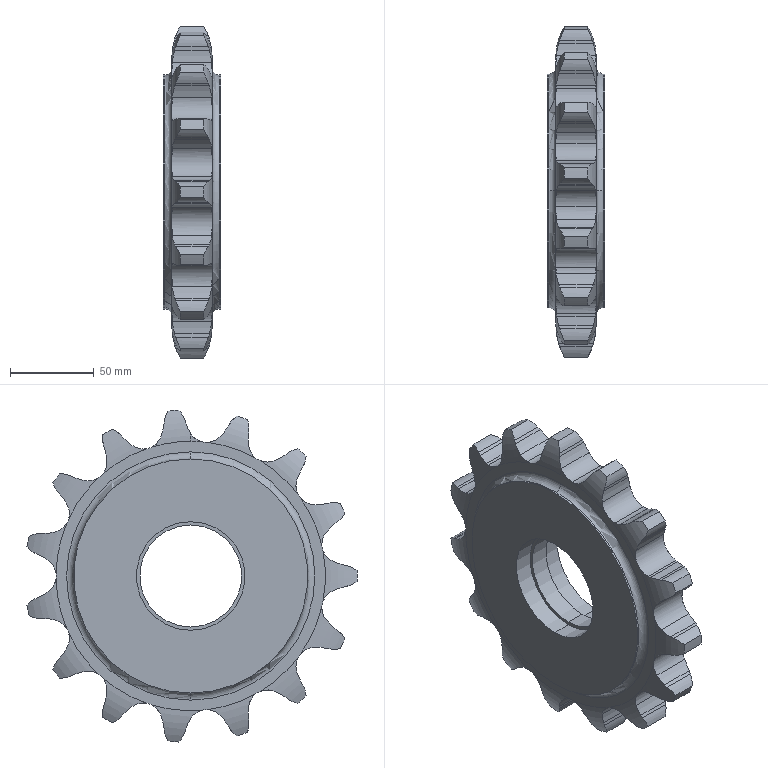Part | SolidWorks | features ICE 4, CirPattern 1, Cut 1, MirrorPattern 1, RefAxis 1, Revolution 1 | 1 solid | 179 faces | box 34.469 x 197.46 x 198.492 mm | volume 635877 mm3 | cylinder 107 | torus 36 | plane 36 | commonest cylinder face diameters 32.838 x32 58.009 x31 22.441 x19 199 x15 65 x4 140 x4